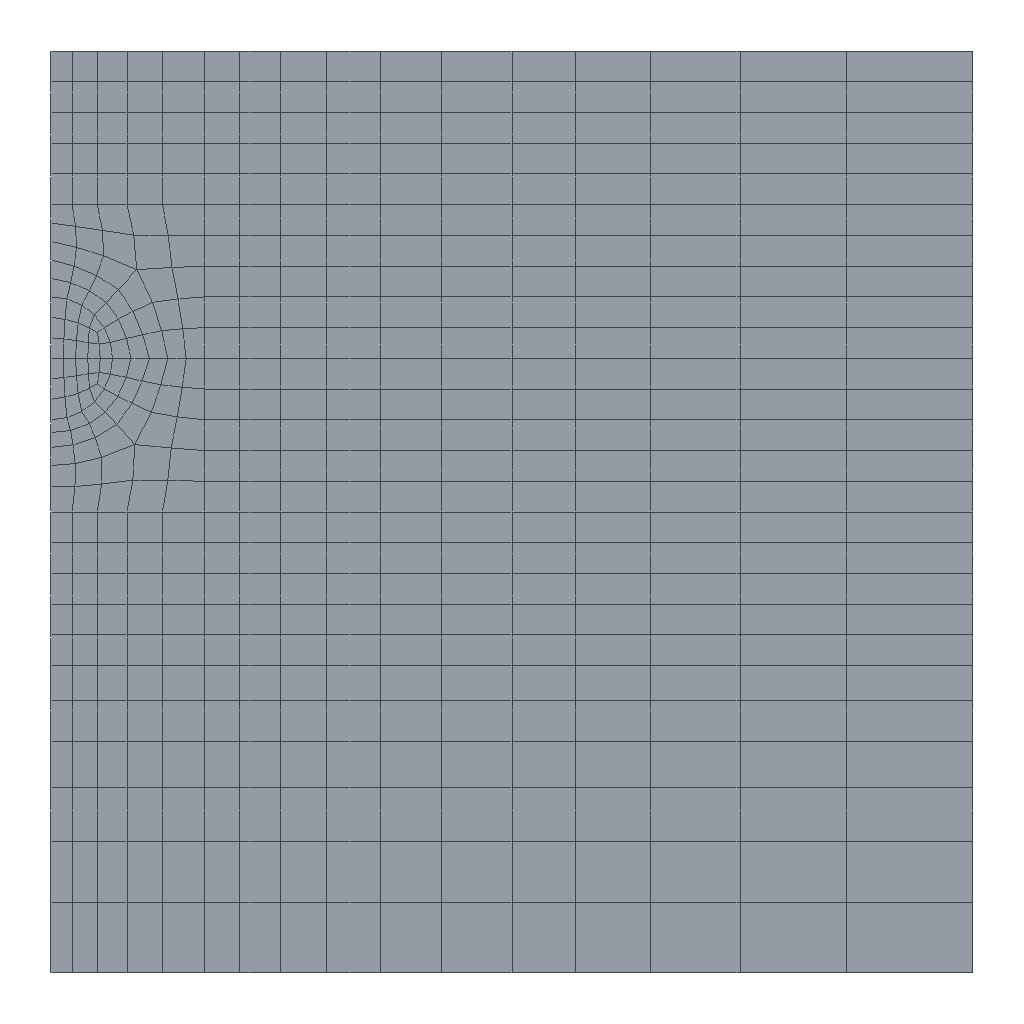Simulation study | abaqus
Set-up summary:
category,name,step,type,value,unit,region
solver,abaqus,,Abaqus/CAE 2024
units,mm-N-s-tonne (MPa),,inferred,E=200000 density=
analysis,geo,,geostatic
analysis,remove,,static,time_period=1
mesh,nodes,,,508
mesh,elements,,,462
element_type,CPE4,,,462
material,soil,,E,200000
material,soil,,nu,0.2
section,soil,,solid section,,,_PickedSet5
load,stress,initial,initial condition stress
load,Load-1,geo,by,-20,,_PickedSet6
load,Load-2,remove,pressure,50,,_PickedSurf10
bc,BC-1,initial,fixed,[dofs=x],,_PickedSet4
bc,BC-2,initial,fixed,"[dofs=x,y n=2]",,_PickedSet5
Abaqus input file, long lists of numbers shortened:
*Heading
** Job name: deck Model name: Model-1
** Generated by: Abaqus/CAE 2024
*Preprint, echo=NO, model=NO, history=NO, contact=NO
**
** PARTS
**
*Part, name=soil
*Node
      1,          60.,         -10.
      2,          30.,         -10.
** (506 more lines like these left out)
*Element, type=CPE4
 1,   1,  28, 208,  43
 2,  28,  29, 209, 208
** (460 more lines like these left out)
*Nset, nset=all, generate
   1,  508,    1
*Elset, elset=all, generate
   1,  462,    1
*Nset, nset=remove
  19,  20,  24,  27, 139, 140, 141, 142, 143, 168, 169, 170, 171, 172, 195, 196
 197, 198, 199, 200, 201, 202, 468, 469, 470, 471, 472, 473, 474, 475, 476, 477
** (1 more lines like these left out)
*Elset, elset=remove, generate
 399,  426,    1
*Nset, nset=_PickedSet5, internal, generate
   1,  508,    1
*Elset, elset=_PickedSet5, internal, generate
   1,  462,    1
** Section: soil
*Solid Section, elset=_PickedSet5, material=soil
1.,
*End Part
**
**
** ASSEMBLY
**
*Assembly, name=Assembly
**
*Instance, name=soil-1, part=soil
*End Instance
**
*Nset, nset=_PickedSet4, internal, instance=soil-1
   1,   4,   7,   8,  10,  11,  14,  20,  21,  22,  23,  24,  26,  27,  40,  41
  42,  43,  53,  54,  55,  56,  57,  70,  71,  72,  73,  96,  97,  98,  99, 127
** (2 more lines like these left out)
*Elset, elset=_PickedSet4, internal, instance=soil-1
   1,   6,  11,  16,  21,  50,  51,  52,  53,  54,  55,  76,  77,  78,  79,  80
 111, 116, 121, 126, 131, 196, 197, 223, 226, 229, 250, 251, 252, 253, 254, 259
** (2 more lines like these left out)
*Nset, nset=_PickedSet5, internal, instance=soil-1
   5,   8,  25,  26,  58,  59,  60,  61, 186, 187, 188, 189, 203, 204, 205, 206
 207,
*Elset, elset=_PickedSet5, internal, instance=soil-1
  26,  32,  38,  44,  50, 364, 365, 366, 367, 368, 432, 438, 444, 450, 456, 462
*Nset, nset=_PickedSet6, internal, instance=soil-1, generate
   1,  508,    1
*Elset, elset=_PickedSet6, internal, instance=soil-1, generate
   1,  462,    1
*Nset, nset=_PickedSet7, internal, instance=soil-1, generate
   1,  508,    1
*Elset, elset=_PickedSet7, internal, instance=soil-1, generate
   1,  462,    1
*Elset, elset=__PickedSurf10_S4, internal, instance=soil-1, generate
 166,  191,    5
*Elset, elset=__PickedSurf10_S2, internal, instance=soil-1, generate
 234,  254,    5
*Surface, type=ELEMENT, name=_PickedSurf10, internal
__PickedSurf10_S4, S4
__PickedSurf10_S2, S2
*End Assembly
**
** MATERIALS
**
*Material, name=soil
*Elastic
200000., 0.2
**
** BOUNDARY CONDITIONS
**
** Name: BC-1 Type: Displacement/Rotation
*Boundary
_PickedSet4, 1, 1
** Name: BC-2 Type: Displacement/Rotation
*Boundary
_PickedSet5, 1, 1
_PickedSet5, 2, 2
**
** PREDEFINED FIELDS
**
** Name: stress   Type: Geostatic stress
*Initial Conditions, type=STRESS, GEOSTATIC
_PickedSet7, 0., 20., -1200., -40., 0.5, 0.5
** ----------------------------------------------------------------
**
** STEP: geo
**
*Step, name=geo, nlgeom=NO
*Geostatic
**
** LOADS
**
** Name: Load-1   Type: Body force
*Dload
_PickedSet6, BY, -20.
**
** OUTPUT REQUESTS
**
*Restart, write, frequency=0
*Print, solve=NO
**
** FIELD OUTPUT: F-Output-1
**
*Output, field, variable=PRESELECT
**
** HISTORY OUTPUT: H-Output-1
**
*Output, history, variable=PRESELECT
*End Step
** ----------------------------------------------------------------
**
** STEP: remove
**
*Step, name=remove, nlgeom=NO
*Static
0.1, 1., 1e-05, 0.2
**
** LOADS
**
** Name: Load-2   Type: Pressure
*Dsload
_PickedSurf10, P, 50.
**
** INTERACTIONS
**
** Interaction: Int-1
*Model Change, remove
soil-1.remove,
**
** OUTPUT REQUESTS
**
*Restart, write, frequency=0
**
** FIELD OUTPUT: F-Output-1
**
*Output, field, variable=PRESELECT
**
** HISTORY OUTPUT: H-Output-1
**
*Output, history, variable=PRESELECT
*End Step
Results summary:
result,odb.job_status,,,JOB_STATUS_COMPLETED_SUCCESSFULLY,"consistent, unstated (Abaqus has no unit system)"
result,steps[0].procedure,geo,,*GEOSTATIC,"consistent, unstated (Abaqus has no unit system)"
result,steps[0].time_period,geo,,1,"consistent, unstated (Abaqus has no unit system)"
result,steps[0].n_frames,geo,,2,"consistent, unstated (Abaqus has no unit system)"
result,steps[0].last_frame.id,geo,,1,"consistent, unstated (Abaqus has no unit system)"
result,steps[0].last_frame.value,geo,,1,"consistent, unstated (Abaqus has no unit system)"
result,steps[0].last_frame.description,geo,,Increment      1: Step Time =    1.000,"consistent, unstated (Abaqus has no unit system)"
result,steps[0].completed,geo,,True,"consistent, unstated (Abaqus has no unit system)"
result,steps[0].max_U_magnitude,geo,,2.20266e-05,"consistent, unstated (Abaqus has no unit system)"
result,steps[0].max_S_mises,geo,,577.081,"consistent, unstated (Abaqus has no unit system)"
result,steps[0].RF_sum[1],geo,,-0.0007444,"consistent, unstated (Abaqus has no unit system)"
result,steps[0].RF_sum[2],geo,,72000,"consistent, unstated (Abaqus has no unit system)"
result,steps[1].procedure,remove,,*STATIC,"consistent, unstated (Abaqus has no unit system)"
result,steps[1].time_period,remove,,1,"consistent, unstated (Abaqus has no unit system)"
result,steps[1].n_frames,remove,,8,"consistent, unstated (Abaqus has no unit system)"
result,steps[1].last_frame.id,remove,,7,"consistent, unstated (Abaqus has no unit system)"
result,steps[1].last_frame.value,remove,,1,"consistent, unstated (Abaqus has no unit system)"
result,steps[1].last_frame.description,remove,,Increment      7: Step Time =    1.000,"consistent, unstated (Abaqus has no unit system)"
result,steps[1].completed,remove,,True,"consistent, unstated (Abaqus has no unit system)"
result,steps[1].max_U_magnitude,remove,,0.02076,"consistent, unstated (Abaqus has no unit system)"
result,steps[1].max_S_mises,remove,,842.783,"consistent, unstated (Abaqus has no unit system)"
result,steps[1].RF_sum[1],remove,,0.0007759,"consistent, unstated (Abaqus has no unit system)"
result,steps[1].RF_sum[2],remove,,73003.1,"consistent, unstated (Abaqus has no unit system)"